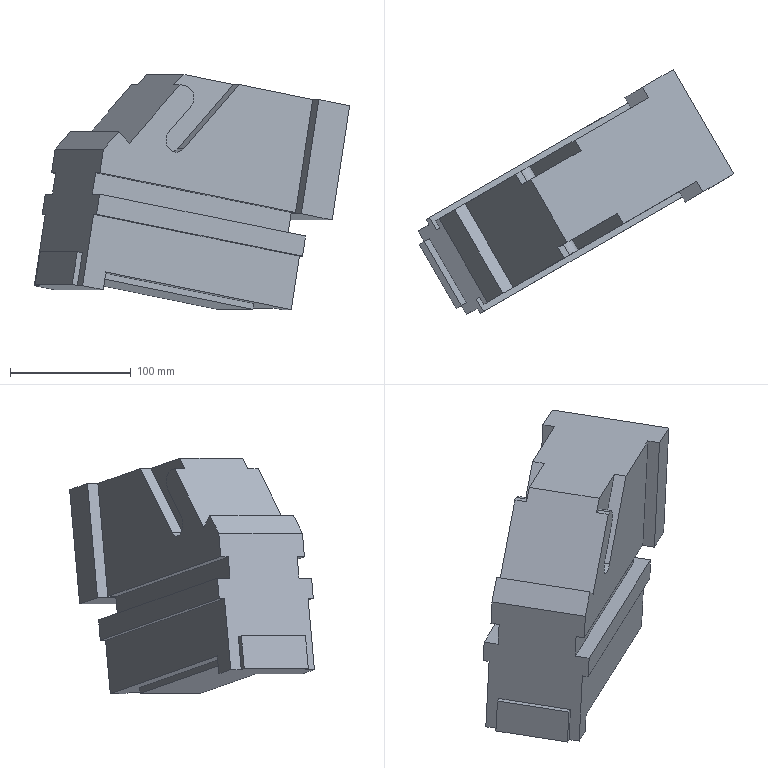Part | NX | features solid 2 | 1 solid | 55 faces | box 261.204 x 202.768 x 194.943 mm | volume 2714300 mm3 | plane 50 | cylinder 5 | commonest cylinder face diameters 20 x5